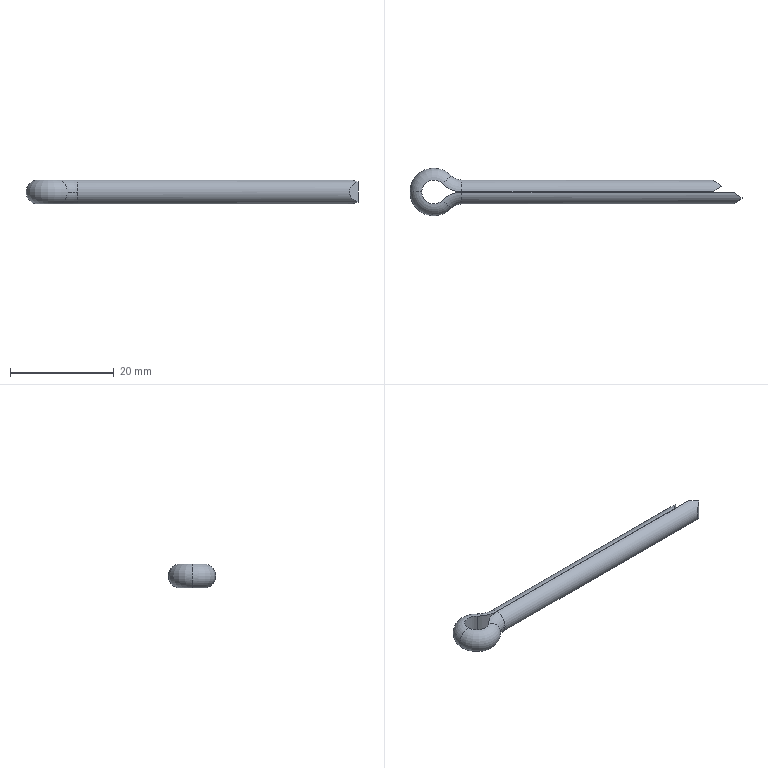Part | SolidWorks | features ICE 1, Sweep 1 | 1 solid | 18 faces | box 64 x 9.2 x 4.6 mm | volume 1032 mm3 | torus 6 | cylinder 6 | plane 6 | commonest cylinder face diameters 4.6 x3 10.358 x2 4.62 x1
STEP:
#1=CARTESIAN_POINT('',(5.4,0.01,2.3));
#2=VERTEX_POINT('',#1);
#3=CARTESIAN_POINT('',(5.4,2.3,0.));
#4=VERTEX_POINT('',#3);
#5=CARTESIAN_POINT('',(5.4,0.,0.));
#6=DIRECTION('',(-1.,0.,0.));
#7=DIRECTION('',(0.,0.,1.));
#8=AXIS2_PLACEMENT_3D('',#5,#6,#7);
#9=CIRCLE('',#8,2.3);
#10=EDGE_CURVE('',#2,#4,#9,.T.);
#11=ORIENTED_EDGE('',*,*,#10,.T.);
#12=CARTESIAN_POINT('',(3.317,3.187,0.));
#13=VERTEX_POINT('',#12);
#14=CARTESIAN_POINT('',(5.4,5.189,0.));
#15=DIRECTION('',(0.,0.,-1.));
#16=DIRECTION('',(-1.,0.,0.));
#17=AXIS2_PLACEMENT_3D('',#14,#15,#16);
#18=CIRCLE('',#17,2.889);
#19=EDGE_CURVE('',#4,#13,#18,.T.);
#20=ORIENTED_EDGE('',*,*,#19,.T.);
#21=CARTESIAN_POINT('',(1.666,1.601,2.3));
#22=VERTEX_POINT('',#21);
#23=CARTESIAN_POINT('',(1.658,1.594,0.));
#24=DIRECTION('',(-0.6929,0.721,0.));
#25=DIRECTION('',(0.,0.,1.));
#26=AXIS2_PLACEMENT_3D('',#23,#24,#25);
#27=CIRCLE('',#26,2.3);
#28=EDGE_CURVE('',#22,#13,#27,.T.);
#29=ORIENTED_EDGE('',*,*,#28,.F.);
#30=CARTESIAN_POINT('',(5.4,5.189,2.3));
#31=DIRECTION('',(0.,0.,-1.));
#32=DIRECTION('',(-1.,0.,0.));
#33=AXIS2_PLACEMENT_3D('',#30,#31,#32);
#34=CIRCLE('',#33,5.179);
#35=EDGE_CURVE('',#2,#22,#34,.T.);
#36=ORIENTED_EDGE('',*,*,#35,.F.);
#37=EDGE_LOOP('',(#11,#20,#29,#36));
#38=FACE_OUTER_BOUND('',#37,.T.);
#39=CARTESIAN_POINT('',(5.4,5.189,0.));
#40=DIRECTION('',(0.,0.,-1.));
#41=DIRECTION('',(-1.,0.,0.));
#42=AXIS2_PLACEMENT_3D('',#39,#40,#41);
#43=TOROIDAL_SURFACE('',#42,5.189,2.3);
#44=ADVANCED_FACE('',(#38),#43,.T.);
#45=CARTESIAN_POINT('',(1.666,-1.601,2.3));
#46=VERTEX_POINT('',#45);
#47=CARTESIAN_POINT('',(3.317,-3.187,0.));
#48=VERTEX_POINT('',#47);
#49=CARTESIAN_POINT('',(1.658,-1.594,0.));
#50=DIRECTION('',(0.6929,0.721,0.));
#51=DIRECTION('',(0.,0.,1.));
#52=AXIS2_PLACEMENT_3D('',#49,#50,#51);
#53=CIRCLE('',#52,2.3);
#54=EDGE_CURVE('',#46,#48,#53,.T.);
#55=ORIENTED_EDGE('',*,*,#54,.T.);
#56=CARTESIAN_POINT('',(5.4,-2.3,0.));
#57=VERTEX_POINT('',#56);
#58=CARTESIAN_POINT('',(5.4,-5.189,0.));
#59=DIRECTION('',(0.,0.,-1.));
#60=DIRECTION('',(-1.,0.,0.));
#61=AXIS2_PLACEMENT_3D('',#58,#59,#60);
#62=CIRCLE('',#61,2.889);
#63=EDGE_CURVE('',#48,#57,#62,.T.);
#64=ORIENTED_EDGE('',*,*,#63,.T.);
#65=CARTESIAN_POINT('',(5.4,-0.01,2.3));
#66=VERTEX_POINT('',#65);
#67=CARTESIAN_POINT('',(5.4,0.,0.));
#68=DIRECTION('',(1.,0.,0.));
#69=DIRECTION('',(0.,0.,1.));
#70=AXIS2_PLACEMENT_3D('',#67,#68,#69);
#71=CIRCLE('',#70,2.3);
#72=EDGE_CURVE('',#66,#57,#71,.T.);
#73=ORIENTED_EDGE('',*,*,#72,.F.);
#74=CARTESIAN_POINT('',(5.4,-5.189,2.3));
#75=DIRECTION('',(0.,0.,-1.));
#76=DIRECTION('',(-1.,0.,0.));
#77=AXIS2_PLACEMENT_3D('',#74,#75,#76);
#78=CIRCLE('',#77,5.179);
#79=EDGE_CURVE('',#46,#66,#78,.T.);
#80=ORIENTED_EDGE('',*,*,#79,.F.);
#81=EDGE_LOOP('',(#55,#64,#73,#80));
#82=FACE_OUTER_BOUND('',#81,.T.);
#83=CARTESIAN_POINT('',(5.4,-5.189,0.));
#84=DIRECTION('',(0.,0.,-1.));
#85=DIRECTION('',(-1.,0.,0.));
#86=AXIS2_PLACEMENT_3D('',#83,#84,#85);
#87=TOROIDAL_SURFACE('',#86,5.189,2.3);
#88=ADVANCED_FACE('',(#82),#87,.T.);
#89=CARTESIAN_POINT('',(5.4,0.01,-2.3));
#90=VERTEX_POINT('',#89);
#91=CARTESIAN_POINT('',(5.4,0.,0.));
#92=DIRECTION('',(-1.,0.,0.));
#93=DIRECTION('',(0.,0.,1.));
#94=AXIS2_PLACEMENT_3D('',#91,#92,#93);
#95=CIRCLE('',#94,2.3);
#96=EDGE_CURVE('',#4,#90,#95,.T.);
#97=ORIENTED_EDGE('',*,*,#96,.F.);
#98=CARTESIAN_POINT('',(53.761,2.3,0.));
#99=VERTEX_POINT('',#98);
#100=CARTESIAN_POINT('',(5.4,2.3,0.));
#101=DIRECTION('',(1.,0.,0.));
#102=VECTOR('',#101,1000.);
#103=LINE('',#100,#102);
#104=EDGE_CURVE('',#4,#99,#103,.T.);
#105=ORIENTED_EDGE('',*,*,#104,.T.);
#106=CARTESIAN_POINT('',(55.4,1.145,-1.995));
#107=VERTEX_POINT('',#106);
#108=CARTESIAN_POINT('',(53.761,2.3,0.));
#109=CARTESIAN_POINT('',(53.761,2.3,-0.8441));
#110=CARTESIAN_POINT('',(54.361,1.877,-1.575));
#111=CARTESIAN_POINT('',(55.4,1.145,-1.995));
#112=(BOUNDED_CURVE()B_SPLINE_CURVE(3,(#108,#109,#110,#111),.UNSPECIFIED.,.F.,.F.)B_SPLINE_CURVE_WITH_KNOTS((4,4),(3.142,4.191),.UNSPECIFIED.)CURVE()GEOMETRIC_REPRESENTATION_ITEM()RATIONAL_B_SPLINE_CURVE((1.,0.9103,0.9103,1.))REPRESENTATION_ITEM(''));
#113=EDGE_CURVE('',#99,#107,#112,.T.);
#114=ORIENTED_EDGE('',*,*,#113,.T.);
#115=CARTESIAN_POINT('',(53.769,0.01,-2.3));
#116=VERTEX_POINT('',#115);
#117=CARTESIAN_POINT('',(55.4,1.145,-1.995));
#118=CARTESIAN_POINT('',(54.901,0.7975,-2.194));
#119=CARTESIAN_POINT('',(54.344,0.4106,-2.298));
#120=CARTESIAN_POINT('',(53.769,0.01,-2.3));
#121=(BOUNDED_CURVE()B_SPLINE_CURVE(3,(#117,#118,#119,#120),.UNSPECIFIED.,.F.,.T.)B_SPLINE_CURVE_WITH_KNOTS((4,4),(1.05,1.566),.UNSPECIFIED.)CURVE()GEOMETRIC_REPRESENTATION_ITEM()RATIONAL_B_SPLINE_CURVE((1.,0.9779,0.9779,1.))REPRESENTATION_ITEM(''));
#122=EDGE_CURVE('',#107,#116,#121,.T.);
#123=ORIENTED_EDGE('',*,*,#122,.T.);
#124=CARTESIAN_POINT('',(5.4,0.01,-2.3));
#125=DIRECTION('',(1.,0.,0.));
#126=VECTOR('',#125,1000.);
#127=LINE('',#124,#126);
#128=EDGE_CURVE('',#90,#116,#127,.T.);
#129=ORIENTED_EDGE('',*,*,#128,.F.);
#130=EDGE_LOOP('',(#97,#105,#114,#123,#129));
#131=FACE_OUTER_BOUND('',#130,.T.);
#132=CARTESIAN_POINT('',(5.4,0.,0.));
#133=DIRECTION('',(1.,0.,0.));
#134=DIRECTION('',(0.,1.,0.));
#135=AXIS2_PLACEMENT_3D('',#132,#133,#134);
#136=CYLINDRICAL_SURFACE('',#135,2.3);
#137=ADVANCED_FACE('',(#131),#136,.T.);
#138=CARTESIAN_POINT('',(1.666,1.601,-2.3));
#139=VERTEX_POINT('',#138);
#140=CARTESIAN_POINT('',(-2.31,0.,-2.3));
#141=VERTEX_POINT('',#140);
#142=CARTESIAN_POINT('',(0.,0.,-2.3));
#143=DIRECTION('',(0.,0.,1.));
#144=DIRECTION('',(1.,0.,0.));
#145=AXIS2_PLACEMENT_3D('',#142,#143,#144);
#146=CIRCLE('',#145,2.31);
#147=EDGE_CURVE('',#139,#141,#146,.T.);
#148=ORIENTED_EDGE('',*,*,#147,.T.);
#149=CARTESIAN_POINT('',(-2.31,0.,2.3));
#150=VERTEX_POINT('',#149);
#151=CARTESIAN_POINT('',(-2.3,0.,0.));
#152=DIRECTION('',(0.,1.,0.));
#153=DIRECTION('',(-1.,0.,0.));
#154=AXIS2_PLACEMENT_3D('',#151,#152,#153);
#155=CIRCLE('',#154,2.3);
#156=EDGE_CURVE('',#141,#150,#155,.T.);
#157=ORIENTED_EDGE('',*,*,#156,.T.);
#158=CARTESIAN_POINT('',(0.,0.,2.3));
#159=DIRECTION('',(0.,0.,1.));
#160=DIRECTION('',(1.,0.,0.));
#161=AXIS2_PLACEMENT_3D('',#158,#159,#160);
#162=CIRCLE('',#161,2.31);
#163=EDGE_CURVE('',#22,#150,#162,.T.);
#164=ORIENTED_EDGE('',*,*,#163,.F.);
#165=ORIENTED_EDGE('',*,*,#28,.T.);
#166=CARTESIAN_POINT('',(1.658,1.594,0.));
#167=DIRECTION('',(-0.6929,0.721,0.));
#168=DIRECTION('',(0.,0.,1.));
#169=AXIS2_PLACEMENT_3D('',#166,#167,#168);
#170=CIRCLE('',#169,2.3);
#171=EDGE_CURVE('',#13,#139,#170,.T.);
#172=ORIENTED_EDGE('',*,*,#171,.T.);
#173=EDGE_LOOP('',(#148,#157,#164,#165,#172));
#174=FACE_OUTER_BOUND('',#173,.T.);
#175=CARTESIAN_POINT('',(0.,0.,0.));
#176=DIRECTION('',(0.,0.,1.));
#177=DIRECTION('',(1.,0.,0.));
#178=AXIS2_PLACEMENT_3D('',#175,#176,#177);
#179=TOROIDAL_SURFACE('',#178,2.3,2.3);
#180=ADVANCED_FACE('',(#174),#179,.T.);
#181=CARTESIAN_POINT('',(59.4,-1.155,-1.989));
#182=VERTEX_POINT('',#181);
#183=CARTESIAN_POINT('',(57.775,-0.01,-2.3));
#184=VERTEX_POINT('',#183);
#185=CARTESIAN_POINT('',(59.4,-1.155,-1.989));
#186=CARTESIAN_POINT('',(58.904,-0.8051,-2.192));
#187=CARTESIAN_POINT('',(58.349,-0.4146,-2.298));
#188=CARTESIAN_POINT('',(57.775,-0.01,-2.3));
#189=(BOUNDED_CURVE()B_SPLINE_CURVE(3,(#185,#186,#187,#188),.UNSPECIFIED.,.F.,.F.)B_SPLINE_CURVE_WITH_KNOTS((4,4),(1.045,1.566),.UNSPECIFIED.)CURVE()GEOMETRIC_REPRESENTATION_ITEM()RATIONAL_B_SPLINE_CURVE((1.,0.9774,0.9774,1.))REPRESENTATION_ITEM(''));
#190=EDGE_CURVE('',#182,#184,#189,.T.);
#191=ORIENTED_EDGE('',*,*,#190,.F.);
#192=CARTESIAN_POINT('',(59.4,-1.155,1.989));
#193=VERTEX_POINT('',#192);
#194=CARTESIAN_POINT('',(59.4,-1.155,1.989));
#195=CARTESIAN_POINT('',(56.933,-2.871,0.9923));
#196=CARTESIAN_POINT('',(56.933,-2.871,-0.9923));
#197=CARTESIAN_POINT('',(59.4,-1.155,-1.989));
#198=(BOUNDED_CURVE()B_SPLINE_CURVE(3,(#194,#195,#196,#197),.UNSPECIFIED.,.F.,.F.)B_SPLINE_CURVE_WITH_KNOTS((4,4),(2.097,4.186),.UNSPECIFIED.)CURVE()GEOMETRIC_REPRESENTATION_ITEM()RATIONAL_B_SPLINE_CURVE((1.,0.6681,0.6681,1.))REPRESENTATION_ITEM(''));
#199=EDGE_CURVE('',#193,#182,#198,.T.);
#200=ORIENTED_EDGE('',*,*,#199,.F.);
#201=CARTESIAN_POINT('',(57.775,-0.01,2.3));
#202=VERTEX_POINT('',#201);
#203=CARTESIAN_POINT('',(57.775,-0.01,2.3));
#204=CARTESIAN_POINT('',(58.349,-0.4146,2.298));
#205=CARTESIAN_POINT('',(58.904,-0.8051,2.192));
#206=CARTESIAN_POINT('',(59.4,-1.155,1.989));
#207=(BOUNDED_CURVE()B_SPLINE_CURVE(3,(#203,#204,#205,#206),.UNSPECIFIED.,.F.,.F.)B_SPLINE_CURVE_WITH_KNOTS((4,4),(4.717,5.238),.UNSPECIFIED.)CURVE()GEOMETRIC_REPRESENTATION_ITEM()RATIONAL_B_SPLINE_CURVE((1.,0.9774,0.9774,1.))REPRESENTATION_ITEM(''));
#208=EDGE_CURVE('',#202,#193,#207,.T.);
#209=ORIENTED_EDGE('',*,*,#208,.F.);
#210=CARTESIAN_POINT('',(5.4,-0.01,2.3));
#211=DIRECTION('',(1.,0.,0.));
#212=VECTOR('',#211,1000.);
#213=LINE('',#210,#212);
#214=EDGE_CURVE('',#66,#202,#213,.T.);
#215=ORIENTED_EDGE('',*,*,#214,.F.);
#216=ORIENTED_EDGE('',*,*,#72,.T.);
#217=CARTESIAN_POINT('',(5.4,-0.01,-2.3));
#218=VERTEX_POINT('',#217);
#219=CARTESIAN_POINT('',(5.4,0.,0.));
#220=DIRECTION('',(1.,0.,0.));
#221=DIRECTION('',(0.,0.,1.));
#222=AXIS2_PLACEMENT_3D('',#219,#220,#221);
#223=CIRCLE('',#222,2.3);
#224=EDGE_CURVE('',#57,#218,#223,.T.);
#225=ORIENTED_EDGE('',*,*,#224,.T.);
#226=CARTESIAN_POINT('',(5.4,-0.01,-2.3));
#227=DIRECTION('',(1.,0.,0.));
#228=VECTOR('',#227,1000.);
#229=LINE('',#226,#228);
#230=EDGE_CURVE('',#218,#184,#229,.T.);
#231=ORIENTED_EDGE('',*,*,#230,.T.);
#232=EDGE_LOOP('',(#191,#200,#209,#215,#216,#225,#231));
#233=FACE_OUTER_BOUND('',#232,.T.);
#234=CARTESIAN_POINT('',(5.4,0.,0.));
#235=DIRECTION('',(1.,0.,0.));
#236=DIRECTION('',(0.,1.,0.));
#237=AXIS2_PLACEMENT_3D('',#234,#235,#236);
#238=CYLINDRICAL_SURFACE('',#237,2.3);
#239=ADVANCED_FACE('',(#233),#238,.T.);
#240=CARTESIAN_POINT('',(57.775,-0.01,-2.3));
#241=DIRECTION('',(0.,0.,1.));
#242=VECTOR('',#241,1000.);
#243=LINE('',#240,#242);
#244=EDGE_CURVE('',#184,#202,#243,.T.);
#245=ORIENTED_EDGE('',*,*,#244,.F.);
#246=ORIENTED_EDGE('',*,*,#230,.F.);
#247=CARTESIAN_POINT('',(5.4,-0.01,-2.3));
#248=DIRECTION('',(0.,0.,1.));
#249=VECTOR('',#248,1000.);
#250=LINE('',#247,#249);
#251=EDGE_CURVE('',#218,#66,#250,.T.);
#252=ORIENTED_EDGE('',*,*,#251,.T.);
#253=ORIENTED_EDGE('',*,*,#214,.T.);
#254=EDGE_LOOP('',(#245,#246,#252,#253));
#255=FACE_OUTER_BOUND('',#254,.T.);
#256=CARTESIAN_POINT('',(5.4,-0.01,-2.3));
#257=DIRECTION('',(0.,1.,0.));
#258=DIRECTION('',(-1.,0.,0.));
#259=AXIS2_PLACEMENT_3D('',#256,#257,#258);
#260=PLANE('',#259);
#261=ADVANCED_FACE('',(#255),#260,.T.);
#262=CARTESIAN_POINT('',(1.666,-1.601,-2.3));
#263=VERTEX_POINT('',#262);
#264=CARTESIAN_POINT('',(1.666,-1.601,-2.3));
#265=DIRECTION('',(0.,0.,1.));
#266=VECTOR('',#265,1000.);
#267=LINE('',#264,#266);
#268=EDGE_CURVE('',#263,#46,#267,.T.);
#269=ORIENTED_EDGE('',*,*,#268,.T.);
#270=ORIENTED_EDGE('',*,*,#79,.T.);
#271=ORIENTED_EDGE('',*,*,#251,.F.);
#272=CARTESIAN_POINT('',(5.4,-5.189,-2.3));
#273=DIRECTION('',(0.,0.,-1.));
#274=DIRECTION('',(-1.,0.,0.));
#275=AXIS2_PLACEMENT_3D('',#272,#273,#274);
#276=CIRCLE('',#275,5.179);
#277=EDGE_CURVE('',#263,#218,#276,.T.);
#278=ORIENTED_EDGE('',*,*,#277,.F.);
#279=EDGE_LOOP('',(#269,#270,#271,#278));
#280=FACE_OUTER_BOUND('',#279,.T.);
#281=CARTESIAN_POINT('',(5.4,-5.189,0.));
#282=DIRECTION('',(0.,0.,-1.));
#283=DIRECTION('',(-1.,0.,0.));
#284=AXIS2_PLACEMENT_3D('',#281,#282,#283);
#285=CYLINDRICAL_SURFACE('',#284,5.179);
#286=ADVANCED_FACE('',(#280),#285,.T.);
#287=ORIENTED_EDGE('',*,*,#63,.F.);
#288=CARTESIAN_POINT('',(1.658,-1.594,0.));
#289=DIRECTION('',(0.6929,0.721,0.));
#290=DIRECTION('',(0.,0.,1.));
#291=AXIS2_PLACEMENT_3D('',#288,#289,#290);
#292=CIRCLE('',#291,2.3);
#293=EDGE_CURVE('',#48,#263,#292,.T.);
#294=ORIENTED_EDGE('',*,*,#293,.T.);
#295=ORIENTED_EDGE('',*,*,#277,.T.);
#296=ORIENTED_EDGE('',*,*,#224,.F.);
#297=EDGE_LOOP('',(#287,#294,#295,#296));
#298=FACE_OUTER_BOUND('',#297,.T.);
#299=CARTESIAN_POINT('',(5.4,-5.189,0.));
#300=DIRECTION('',(0.,0.,-1.));
#301=DIRECTION('',(-1.,0.,0.));
#302=AXIS2_PLACEMENT_3D('',#299,#300,#301);
#303=TOROIDAL_SURFACE('',#302,5.189,2.3);
#304=ADVANCED_FACE('',(#298),#303,.T.);
#305=CARTESIAN_POINT('',(1.666,1.601,-2.3));
#306=DIRECTION('',(0.,0.,1.));
#307=VECTOR('',#306,1000.);
#308=LINE('',#305,#307);
#309=EDGE_CURVE('',#139,#22,#308,.T.);
#310=ORIENTED_EDGE('',*,*,#309,.T.);
#311=ORIENTED_EDGE('',*,*,#163,.T.);
#312=CARTESIAN_POINT('',(0.,0.,2.3));
#313=DIRECTION('',(0.,0.,1.));
#314=DIRECTION('',(1.,0.,0.));
#315=AXIS2_PLACEMENT_3D('',#312,#313,#314);
#316=CIRCLE('',#315,2.31);
#317=EDGE_CURVE('',#150,#46,#316,.T.);
#318=ORIENTED_EDGE('',*,*,#317,.T.);
#319=ORIENTED_EDGE('',*,*,#268,.F.);
#320=CARTESIAN_POINT('',(0.,0.,-2.3));
#321=DIRECTION('',(0.,0.,1.));
#322=DIRECTION('',(1.,0.,0.));
#323=AXIS2_PLACEMENT_3D('',#320,#321,#322);
#324=CIRCLE('',#323,2.31);
#325=EDGE_CURVE('',#141,#263,#324,.T.);
#326=ORIENTED_EDGE('',*,*,#325,.F.);
#327=ORIENTED_EDGE('',*,*,#147,.F.);
#328=EDGE_LOOP('',(#310,#311,#318,#319,#326,#327));
#329=FACE_OUTER_BOUND('',#328,.T.);
#330=CARTESIAN_POINT('',(0.,0.,0.));
#331=DIRECTION('',(0.,0.,1.));
#332=DIRECTION('',(1.,0.,0.));
#333=AXIS2_PLACEMENT_3D('',#330,#331,#332);
#334=CYLINDRICAL_SURFACE('',#333,2.31);
#335=ADVANCED_FACE('',(#329),#334,.F.);
#336=ORIENTED_EDGE('',*,*,#156,.F.);
#337=ORIENTED_EDGE('',*,*,#325,.T.);
#338=ORIENTED_EDGE('',*,*,#293,.F.);
#339=ORIENTED_EDGE('',*,*,#54,.F.);
#340=ORIENTED_EDGE('',*,*,#317,.F.);
#341=EDGE_LOOP('',(#336,#337,#338,#339,#340));
#342=FACE_OUTER_BOUND('',#341,.T.);
#343=CARTESIAN_POINT('',(0.,0.,0.));
#344=DIRECTION('',(0.,0.,1.));
#345=DIRECTION('',(1.,0.,0.));
#346=AXIS2_PLACEMENT_3D('',#343,#344,#345);
#347=TOROIDAL_SURFACE('',#346,2.3,2.3);
#348=ADVANCED_FACE('',(#342),#347,.T.);
#349=CARTESIAN_POINT('',(5.4,0.01,-2.3));
#350=DIRECTION('',(0.,0.,1.));
#351=VECTOR('',#350,1000.);
#352=LINE('',#349,#351);
#353=EDGE_CURVE('',#90,#2,#352,.T.);
#354=ORIENTED_EDGE('',*,*,#353,.T.);
#355=ORIENTED_EDGE('',*,*,#35,.T.);
#356=ORIENTED_EDGE('',*,*,#309,.F.);
#357=CARTESIAN_POINT('',(5.4,5.189,-2.3));
#358=DIRECTION('',(0.,0.,-1.));
#359=DIRECTION('',(-1.,0.,0.));
#360=AXIS2_PLACEMENT_3D('',#357,#358,#359);
#361=CIRCLE('',#360,5.179);
#362=EDGE_CURVE('',#90,#139,#361,.T.);
#363=ORIENTED_EDGE('',*,*,#362,.F.);
#364=EDGE_LOOP('',(#354,#355,#356,#363));
#365=FACE_OUTER_BOUND('',#364,.T.);
#366=CARTESIAN_POINT('',(5.4,5.189,0.));
#367=DIRECTION('',(0.,0.,-1.));
#368=DIRECTION('',(-1.,0.,0.));
#369=AXIS2_PLACEMENT_3D('',#366,#367,#368);
#370=CYLINDRICAL_SURFACE('',#369,5.179);
#371=ADVANCED_FACE('',(#365),#370,.T.);
#372=ORIENTED_EDGE('',*,*,#19,.F.);
#373=ORIENTED_EDGE('',*,*,#96,.T.);
#374=ORIENTED_EDGE('',*,*,#362,.T.);
#375=ORIENTED_EDGE('',*,*,#171,.F.);
#376=EDGE_LOOP('',(#372,#373,#374,#375));
#377=FACE_OUTER_BOUND('',#376,.T.);
#378=CARTESIAN_POINT('',(5.4,5.189,0.));
#379=DIRECTION('',(0.,0.,-1.));
#380=DIRECTION('',(-1.,0.,0.));
#381=AXIS2_PLACEMENT_3D('',#378,#379,#380);
#382=TOROIDAL_SURFACE('',#381,5.189,2.3);
#383=ADVANCED_FACE('',(#377),#382,.T.);
#384=ORIENTED_EDGE('',*,*,#104,.F.);
#385=ORIENTED_EDGE('',*,*,#10,.F.);
#386=CARTESIAN_POINT('',(53.769,0.01,2.3));
#387=VERTEX_POINT('',#386);
#388=CARTESIAN_POINT('',(5.4,0.01,2.3));
#389=DIRECTION('',(1.,0.,0.));
#390=VECTOR('',#389,1000.);
#391=LINE('',#388,#390);
#392=EDGE_CURVE('',#2,#387,#391,.T.);
#393=ORIENTED_EDGE('',*,*,#392,.T.);
#394=CARTESIAN_POINT('',(55.4,1.145,1.995));
#395=VERTEX_POINT('',#394);
#396=CARTESIAN_POINT('',(53.769,0.01,2.3));
#397=CARTESIAN_POINT('',(54.344,0.4106,2.298));
#398=CARTESIAN_POINT('',(54.901,0.7975,2.194));
#399=CARTESIAN_POINT('',(55.4,1.145,1.995));
#400=(BOUNDED_CURVE()B_SPLINE_CURVE(3,(#396,#397,#398,#399),.UNSPECIFIED.,.F.,.F.)B_SPLINE_CURVE_WITH_KNOTS((4,4),(4.717,5.233),.UNSPECIFIED.)CURVE()GEOMETRIC_REPRESENTATION_ITEM()RATIONAL_B_SPLINE_CURVE((1.,0.9779,0.9779,1.))REPRESENTATION_ITEM(''));
#401=EDGE_CURVE('',#387,#395,#400,.T.);
#402=ORIENTED_EDGE('',*,*,#401,.T.);
#403=CARTESIAN_POINT('',(55.4,1.145,1.995));
#404=CARTESIAN_POINT('',(54.361,1.877,1.575));
#405=CARTESIAN_POINT('',(53.761,2.3,0.8441));
#406=CARTESIAN_POINT('',(53.761,2.3,0.));
#407=(BOUNDED_CURVE()B_SPLINE_CURVE(3,(#403,#404,#405,#406),.UNSPECIFIED.,.F.,.F.)B_SPLINE_CURVE_WITH_KNOTS((4,4),(2.092,3.142),.UNSPECIFIED.)CURVE()GEOMETRIC_REPRESENTATION_ITEM()RATIONAL_B_SPLINE_CURVE((1.,0.9103,0.9103,1.))REPRESENTATION_ITEM(''));
#408=EDGE_CURVE('',#395,#99,#407,.T.);
#409=ORIENTED_EDGE('',*,*,#408,.T.);
#410=EDGE_LOOP('',(#384,#385,#393,#402,#409));
#411=FACE_OUTER_BOUND('',#410,.T.);
#412=CARTESIAN_POINT('',(5.4,0.,0.));
#413=DIRECTION('',(1.,0.,0.));
#414=DIRECTION('',(0.,1.,0.));
#415=AXIS2_PLACEMENT_3D('',#412,#413,#414);
#416=CYLINDRICAL_SURFACE('',#415,2.3);
#417=ADVANCED_FACE('',(#411),#416,.T.);
#418=ORIENTED_EDGE('',*,*,#128,.T.);
#419=CARTESIAN_POINT('',(53.769,0.01,-2.3));
#420=DIRECTION('',(0.,0.,1.));
#421=VECTOR('',#420,1000.);
#422=LINE('',#419,#421);
#423=EDGE_CURVE('',#116,#387,#422,.T.);
#424=ORIENTED_EDGE('',*,*,#423,.T.);
#425=ORIENTED_EDGE('',*,*,#392,.F.);
#426=ORIENTED_EDGE('',*,*,#353,.F.);
#427=EDGE_LOOP('',(#418,#424,#425,#426));
#428=FACE_OUTER_BOUND('',#427,.T.);
#429=CARTESIAN_POINT('',(5.4,0.01,-2.3));
#430=DIRECTION('',(0.,1.,0.));
#431=DIRECTION('',(-1.,0.,0.));
#432=AXIS2_PLACEMENT_3D('',#429,#430,#431);
#433=PLANE('',#432);
#434=ADVANCED_FACE('',(#428),#433,.F.);
#435=CARTESIAN_POINT('',(55.4,1.145,-2.3));
#436=DIRECTION('',(0.,0.,1.));
#437=VECTOR('',#436,1000.);
#438=LINE('',#435,#437);
#439=EDGE_CURVE('',#107,#395,#438,.T.);
#440=ORIENTED_EDGE('',*,*,#439,.T.);
#441=ORIENTED_EDGE('',*,*,#401,.F.);
#442=ORIENTED_EDGE('',*,*,#423,.F.);
#443=ORIENTED_EDGE('',*,*,#122,.F.);
#444=EDGE_LOOP('',(#440,#441,#442,#443));
#445=FACE_OUTER_BOUND('',#444,.T.);
#446=CARTESIAN_POINT('',(55.4,1.145,-2.3));
#447=DIRECTION('',(-0.5711,0.8209,0.));
#448=DIRECTION('',(-0.8209,-0.5711,0.));
#449=AXIS2_PLACEMENT_3D('',#446,#447,#448);
#450=PLANE('',#449);
#451=ADVANCED_FACE('',(#445),#450,.F.);
#452=ORIENTED_EDGE('',*,*,#439,.F.);
#453=ORIENTED_EDGE('',*,*,#113,.F.);
#454=ORIENTED_EDGE('',*,*,#408,.F.);
#455=EDGE_LOOP('',(#452,#453,#454));
#456=FACE_OUTER_BOUND('',#455,.T.);
#457=CARTESIAN_POINT('',(55.4,1.145,-2.3));
#458=DIRECTION('',(-0.5761,-0.8174,0.));
#459=DIRECTION('',(0.8174,-0.5761,0.));
#460=AXIS2_PLACEMENT_3D('',#457,#458,#459);
#461=PLANE('',#460);
#462=ADVANCED_FACE('',(#456),#461,.F.);
#463=ORIENTED_EDGE('',*,*,#199,.T.);
#464=CARTESIAN_POINT('',(59.4,-1.155,-2.3));
#465=DIRECTION('',(0.,0.,1.));
#466=VECTOR('',#465,1000.);
#467=LINE('',#464,#466);
#468=EDGE_CURVE('',#182,#193,#467,.T.);
#469=ORIENTED_EDGE('',*,*,#468,.T.);
#470=EDGE_LOOP('',(#463,#469));
#471=FACE_OUTER_BOUND('',#470,.T.);
#472=CARTESIAN_POINT('',(59.4,-1.155,-2.3));
#473=DIRECTION('',(-0.5711,0.8209,0.));
#474=DIRECTION('',(-0.8209,-0.5711,0.));
#475=AXIS2_PLACEMENT_3D('',#472,#473,#474);
#476=PLANE('',#475);
#477=ADVANCED_FACE('',(#471),#476,.F.);
#478=ORIENTED_EDGE('',*,*,#190,.T.);
#479=ORIENTED_EDGE('',*,*,#244,.T.);
#480=ORIENTED_EDGE('',*,*,#208,.T.);
#481=ORIENTED_EDGE('',*,*,#468,.F.);
#482=EDGE_LOOP('',(#478,#479,#480,#481));
#483=FACE_OUTER_BOUND('',#482,.T.);
#484=CARTESIAN_POINT('',(59.4,-1.155,-2.3));
#485=DIRECTION('',(-0.5761,-0.8174,0.));
#486=DIRECTION('',(0.8174,-0.5761,0.));
#487=AXIS2_PLACEMENT_3D('',#484,#485,#486);
#488=PLANE('',#487);
#489=ADVANCED_FACE('',(#483),#488,.F.);
#490=CLOSED_SHELL('',(#44,#88,#137,#180,#239,#261,#286,#304,#335,#348,#371,#383,#417,#434,#451,#462,#477,#489));
#491=MANIFOLD_SOLID_BREP('',#490);
#492=CARTESIAN_POINT('',(0.,0.,0.));
#493=DIRECTION('',(0.,0.,1.));
#494=DIRECTION('',(1.,0.,0.));
#495=AXIS2_PLACEMENT_3D('',#492,#493,#494);
#496=(LENGTH_UNIT()NAMED_UNIT(*)SI_UNIT(.MILLI.,.METRE.));
#497=UNCERTAINTY_MEASURE_WITH_UNIT(LENGTH_MEASURE(0.00001),#496,'','');
#498=(NAMED_UNIT(*)PLANE_ANGLE_UNIT()SI_UNIT($,.RADIAN.));
#499=(NAMED_UNIT(*)SI_UNIT($,.STERADIAN.)SOLID_ANGLE_UNIT());
#500=(GEOMETRIC_REPRESENTATION_CONTEXT(3)GLOBAL_UNCERTAINTY_ASSIGNED_CONTEXT((#497))GLOBAL_UNIT_ASSIGNED_CONTEXT((#496,#498,#499))REPRESENTATION_CONTEXT('',''));
#501=ADVANCED_BREP_SHAPE_REPRESENTATION('',(#491,#495),#500);